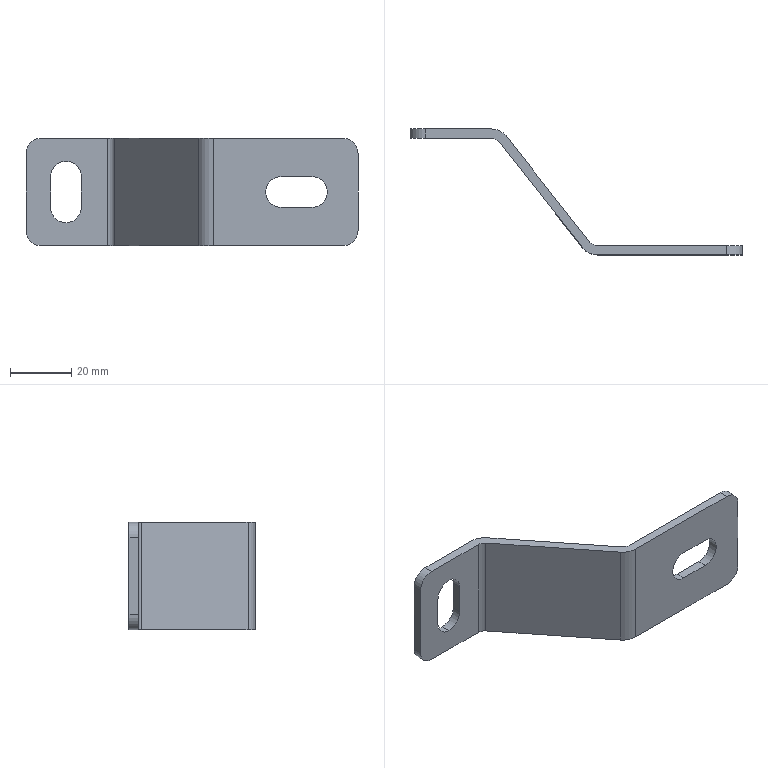Part | STEP file | VD-SYL0380DJ1006_1-4_VD-SYL0380 | 1 solid | 27 faces | box 108 x 41 x 35 mm | volume 12075 mm3 | plane 14 | cylinder 13 | commonest cylinder face diameters 10 x9 6 x2 12 x2
STEP:
#1=CARTESIAN_POINT('',(65.,-38.,-5.));
#2=VERTEX_POINT('',#1);
#3=CARTESIAN_POINT('',(55.,-38.,-5.));
#4=VERTEX_POINT('',#3);
#5=CARTESIAN_POINT('',(65.,-38.,-5.));
#6=DIRECTION('',(-1.,0.,0.));
#7=VECTOR('',#6,1000.);
#8=LINE('',#5,#7);
#9=EDGE_CURVE('',#2,#4,#8,.T.);
#10=ORIENTED_EDGE('',*,*,#9,.F.);
#11=CARTESIAN_POINT('',(65.,-35.,-5.));
#12=VERTEX_POINT('',#11);
#13=CARTESIAN_POINT('',(65.,-35.,-5.));
#14=DIRECTION('',(0.,-1.,0.));
#15=VECTOR('',#14,1000.);
#16=LINE('',#13,#15);
#17=EDGE_CURVE('',#12,#2,#16,.T.);
#18=ORIENTED_EDGE('',*,*,#17,.F.);
#19=CARTESIAN_POINT('',(55.,-35.,-5.));
#20=VERTEX_POINT('',#19);
#21=CARTESIAN_POINT('',(55.,-35.,-5.));
#22=DIRECTION('',(1.,0.,0.));
#23=VECTOR('',#22,1000.);
#24=LINE('',#21,#23);
#25=EDGE_CURVE('',#20,#12,#24,.T.);
#26=ORIENTED_EDGE('',*,*,#25,.F.);
#27=CARTESIAN_POINT('',(55.,-38.,-5.));
#28=DIRECTION('',(0.,1.,0.));
#29=VECTOR('',#28,1000.);
#30=LINE('',#27,#29);
#31=EDGE_CURVE('',#4,#20,#30,.T.);
#32=ORIENTED_EDGE('',*,*,#31,.F.);
#33=EDGE_LOOP('',(#10,#18,#26,#32));
#34=FACE_OUTER_BOUND('',#33,.T.);
#35=CARTESIAN_POINT('',(60.,-36.5,-5.));
#36=DIRECTION('',(0.,0.,1.));
#37=DIRECTION('',(1.,0.,0.));
#38=AXIS2_PLACEMENT_3D('',#35,#36,#37);
#39=PLANE('',#38);
#40=ADVANCED_FACE('',(#34),#39,.T.);
#41=CARTESIAN_POINT('',(55.,-35.,5.));
#42=VERTEX_POINT('',#41);
#43=CARTESIAN_POINT('',(55.,-38.,5.));
#44=VERTEX_POINT('',#43);
#45=CARTESIAN_POINT('',(55.,-35.,5.));
#46=DIRECTION('',(0.,-1.,0.));
#47=VECTOR('',#46,1000.);
#48=LINE('',#45,#47);
#49=EDGE_CURVE('',#42,#44,#48,.T.);
#50=ORIENTED_EDGE('',*,*,#49,.T.);
#51=CARTESIAN_POINT('',(55.,-38.,0.));
#52=DIRECTION('',(0.,1.,0.));
#53=DIRECTION('',(0.,0.,-1.));
#54=AXIS2_PLACEMENT_3D('',#51,#52,#53);
#55=CIRCLE('',#54,5.);
#56=EDGE_CURVE('',#4,#44,#55,.T.);
#57=ORIENTED_EDGE('',*,*,#56,.F.);
#58=ORIENTED_EDGE('',*,*,#31,.T.);
#59=CARTESIAN_POINT('',(55.,-35.,0.));
#60=DIRECTION('',(0.,-1.,0.));
#61=DIRECTION('',(0.,0.,1.));
#62=AXIS2_PLACEMENT_3D('',#59,#60,#61);
#63=CIRCLE('',#62,5.);
#64=EDGE_CURVE('',#42,#20,#63,.T.);
#65=ORIENTED_EDGE('',*,*,#64,.F.);
#66=EDGE_LOOP('',(#50,#57,#58,#65));
#67=FACE_OUTER_BOUND('',#66,.T.);
#68=CARTESIAN_POINT('',(55.,-36.5,0.));
#69=DIRECTION('',(0.,-1.,0.));
#70=DIRECTION('',(0.,0.,-1.));
#71=AXIS2_PLACEMENT_3D('',#68,#69,#70);
#72=CYLINDRICAL_SURFACE('',#71,5.);
#73=ADVANCED_FACE('',(#67),#72,.F.);
#74=CARTESIAN_POINT('',(65.,-38.,5.));
#75=VERTEX_POINT('',#74);
#76=CARTESIAN_POINT('',(55.,-38.,5.));
#77=DIRECTION('',(1.,0.,0.));
#78=VECTOR('',#77,1000.);
#79=LINE('',#76,#78);
#80=EDGE_CURVE('',#44,#75,#79,.T.);
#81=ORIENTED_EDGE('',*,*,#80,.F.);
#82=ORIENTED_EDGE('',*,*,#49,.F.);
#83=CARTESIAN_POINT('',(65.,-35.,5.));
#84=VERTEX_POINT('',#83);
#85=CARTESIAN_POINT('',(65.,-35.,5.));
#86=DIRECTION('',(-1.,0.,0.));
#87=VECTOR('',#86,1000.);
#88=LINE('',#85,#87);
#89=EDGE_CURVE('',#84,#42,#88,.T.);
#90=ORIENTED_EDGE('',*,*,#89,.F.);
#91=CARTESIAN_POINT('',(65.,-38.,5.));
#92=DIRECTION('',(0.,1.,0.));
#93=VECTOR('',#92,1000.);
#94=LINE('',#91,#93);
#95=EDGE_CURVE('',#75,#84,#94,.T.);
#96=ORIENTED_EDGE('',*,*,#95,.F.);
#97=EDGE_LOOP('',(#81,#82,#90,#96));
#98=FACE_OUTER_BOUND('',#97,.T.);
#99=CARTESIAN_POINT('',(60.,-36.5,5.));
#100=DIRECTION('',(0.,0.,-1.));
#101=DIRECTION('',(0.,-1.,0.));
#102=AXIS2_PLACEMENT_3D('',#99,#100,#101);
#103=PLANE('',#102);
#104=ADVANCED_FACE('',(#98),#103,.T.);
#105=ORIENTED_EDGE('',*,*,#17,.T.);
#106=CARTESIAN_POINT('',(65.,-38.,0.));
#107=DIRECTION('',(0.,1.,0.));
#108=DIRECTION('',(0.,0.,1.));
#109=AXIS2_PLACEMENT_3D('',#106,#107,#108);
#110=CIRCLE('',#109,5.);
#111=EDGE_CURVE('',#75,#2,#110,.T.);
#112=ORIENTED_EDGE('',*,*,#111,.F.);
#113=ORIENTED_EDGE('',*,*,#95,.T.);
#114=CARTESIAN_POINT('',(65.,-35.,0.));
#115=DIRECTION('',(0.,-1.,0.));
#116=DIRECTION('',(0.,0.,-1.));
#117=AXIS2_PLACEMENT_3D('',#114,#115,#116);
#118=CIRCLE('',#117,5.);
#119=EDGE_CURVE('',#12,#84,#118,.T.);
#120=ORIENTED_EDGE('',*,*,#119,.F.);
#121=EDGE_LOOP('',(#105,#112,#113,#120));
#122=FACE_OUTER_BOUND('',#121,.T.);
#123=CARTESIAN_POINT('',(65.,-36.5,0.));
#124=DIRECTION('',(0.,-1.,0.));
#125=DIRECTION('',(0.,0.,-1.));
#126=AXIS2_PLACEMENT_3D('',#123,#124,#125);
#127=CYLINDRICAL_SURFACE('',#126,5.);
#128=ADVANCED_FACE('',(#122),#127,.F.);
#129=CARTESIAN_POINT('',(75.,-38.,-17.5));
#130=VERTEX_POINT('',#129);
#131=CARTESIAN_POINT('',(80.,-38.,-12.5));
#132=VERTEX_POINT('',#131);
#133=CARTESIAN_POINT('',(75.,-38.,-12.5));
#134=DIRECTION('',(0.,-1.,0.));
#135=DIRECTION('',(0.,0.,-1.));
#136=AXIS2_PLACEMENT_3D('',#133,#134,#135);
#137=CIRCLE('',#136,5.);
#138=EDGE_CURVE('',#130,#132,#137,.T.);
#139=ORIENTED_EDGE('',*,*,#138,.F.);
#140=CARTESIAN_POINT('',(75.,-35.,-17.5));
#141=VERTEX_POINT('',#140);
#142=CARTESIAN_POINT('',(75.,-38.,-17.5));
#143=DIRECTION('',(0.,1.,0.));
#144=VECTOR('',#143,1000.);
#145=LINE('',#142,#144);
#146=EDGE_CURVE('',#130,#141,#145,.T.);
#147=ORIENTED_EDGE('',*,*,#146,.T.);
#148=CARTESIAN_POINT('',(80.,-35.,-12.5));
#149=VERTEX_POINT('',#148);
#150=CARTESIAN_POINT('',(75.,-35.,-12.5));
#151=DIRECTION('',(0.,1.,0.));
#152=DIRECTION('',(1.,0.,0.));
#153=AXIS2_PLACEMENT_3D('',#150,#151,#152);
#154=CIRCLE('',#153,5.);
#155=EDGE_CURVE('',#149,#141,#154,.T.);
#156=ORIENTED_EDGE('',*,*,#155,.F.);
#157=CARTESIAN_POINT('',(80.,-35.,-12.5));
#158=DIRECTION('',(0.,-1.,0.));
#159=VECTOR('',#158,1000.);
#160=LINE('',#157,#159);
#161=EDGE_CURVE('',#149,#132,#160,.T.);
#162=ORIENTED_EDGE('',*,*,#161,.T.);
#163=EDGE_LOOP('',(#139,#147,#156,#162));
#164=FACE_OUTER_BOUND('',#163,.T.);
#165=CARTESIAN_POINT('',(75.,61.549,-12.5));
#166=DIRECTION('',(0.,-1.,0.));
#167=DIRECTION('',(0.,0.,-1.));
#168=AXIS2_PLACEMENT_3D('',#165,#166,#167);
#169=CYLINDRICAL_SURFACE('',#168,5.);
#170=ADVANCED_FACE('',(#164),#169,.T.);
#171=CARTESIAN_POINT('',(-10.,3.,5.));
#172=VERTEX_POINT('',#171);
#173=CARTESIAN_POINT('',(-20.,3.,5.));
#174=VERTEX_POINT('',#173);
#175=CARTESIAN_POINT('',(-15.,3.,5.));
#176=DIRECTION('',(0.,-1.,0.));
#177=DIRECTION('',(1.,0.,0.));
#178=AXIS2_PLACEMENT_3D('',#175,#176,#177);
#179=CIRCLE('',#178,5.);
#180=EDGE_CURVE('',#172,#174,#179,.T.);
#181=ORIENTED_EDGE('',*,*,#180,.F.);
#182=CARTESIAN_POINT('',(-10.,0.,5.));
#183=VERTEX_POINT('',#182);
#184=CARTESIAN_POINT('',(-10.,3.,5.));
#185=DIRECTION('',(0.,-1.,0.));
#186=VECTOR('',#185,1000.);
#187=LINE('',#184,#186);
#188=EDGE_CURVE('',#172,#183,#187,.T.);
#189=ORIENTED_EDGE('',*,*,#188,.T.);
#190=CARTESIAN_POINT('',(-20.,0.,5.));
#191=VERTEX_POINT('',#190);
#192=CARTESIAN_POINT('',(-15.,0.,5.));
#193=DIRECTION('',(0.,1.,0.));
#194=DIRECTION('',(-1.,0.,0.));
#195=AXIS2_PLACEMENT_3D('',#192,#193,#194);
#196=CIRCLE('',#195,5.);
#197=EDGE_CURVE('',#191,#183,#196,.T.);
#198=ORIENTED_EDGE('',*,*,#197,.F.);
#199=CARTESIAN_POINT('',(-20.,0.,5.));
#200=DIRECTION('',(0.,1.,0.));
#201=VECTOR('',#200,1000.);
#202=LINE('',#199,#201);
#203=EDGE_CURVE('',#191,#174,#202,.T.);
#204=ORIENTED_EDGE('',*,*,#203,.T.);
#205=EDGE_LOOP('',(#181,#189,#198,#204));
#206=FACE_OUTER_BOUND('',#205,.T.);
#207=CARTESIAN_POINT('',(-15.,1.5,5.));
#208=DIRECTION('',(0.,-1.,0.));
#209=DIRECTION('',(0.,0.,-1.));
#210=AXIS2_PLACEMENT_3D('',#207,#208,#209);
#211=CYLINDRICAL_SURFACE('',#210,5.);
#212=ADVANCED_FACE('',(#206),#211,.F.);
#213=CARTESIAN_POINT('',(-20.,0.,-5.));
#214=VERTEX_POINT('',#213);
#215=CARTESIAN_POINT('',(-20.,0.,-5.));
#216=DIRECTION('',(0.,0.,1.));
#217=VECTOR('',#216,1000.);
#218=LINE('',#215,#217);
#219=EDGE_CURVE('',#214,#191,#218,.T.);
#220=ORIENTED_EDGE('',*,*,#219,.F.);
#221=CARTESIAN_POINT('',(-20.,3.,-5.));
#222=VERTEX_POINT('',#221);
#223=CARTESIAN_POINT('',(-20.,3.,-5.));
#224=DIRECTION('',(0.,-1.,0.));
#225=VECTOR('',#224,1000.);
#226=LINE('',#223,#225);
#227=EDGE_CURVE('',#222,#214,#226,.T.);
#228=ORIENTED_EDGE('',*,*,#227,.F.);
#229=CARTESIAN_POINT('',(-20.,3.,5.));
#230=DIRECTION('',(0.,0.,-1.));
#231=VECTOR('',#230,1000.);
#232=LINE('',#229,#231);
#233=EDGE_CURVE('',#174,#222,#232,.T.);
#234=ORIENTED_EDGE('',*,*,#233,.F.);
#235=ORIENTED_EDGE('',*,*,#203,.F.);
#236=EDGE_LOOP('',(#220,#228,#234,#235));
#237=FACE_OUTER_BOUND('',#236,.T.);
#238=CARTESIAN_POINT('',(-20.,1.5,0.));
#239=DIRECTION('',(1.,0.,0.));
#240=DIRECTION('',(0.,1.,0.));
#241=AXIS2_PLACEMENT_3D('',#238,#239,#240);
#242=PLANE('',#241);
#243=ADVANCED_FACE('',(#237),#242,.T.);
#244=CARTESIAN_POINT('',(-15.,3.,-10.));
#245=VERTEX_POINT('',#244);
#246=CARTESIAN_POINT('',(-15.,3.,-5.));
#247=DIRECTION('',(0.,-1.,0.));
#248=DIRECTION('',(-1.,0.,0.));
#249=AXIS2_PLACEMENT_3D('',#246,#247,#248);
#250=CIRCLE('',#249,5.);
#251=EDGE_CURVE('',#222,#245,#250,.T.);
#252=ORIENTED_EDGE('',*,*,#251,.F.);
#253=ORIENTED_EDGE('',*,*,#227,.T.);
#254=CARTESIAN_POINT('',(-15.,0.,-10.));
#255=VERTEX_POINT('',#254);
#256=CARTESIAN_POINT('',(-15.,0.,-5.));
#257=DIRECTION('',(0.,1.,0.));
#258=DIRECTION('',(0.,0.,-1.));
#259=AXIS2_PLACEMENT_3D('',#256,#257,#258);
#260=CIRCLE('',#259,5.);
#261=EDGE_CURVE('',#255,#214,#260,.T.);
#262=ORIENTED_EDGE('',*,*,#261,.F.);
#263=CARTESIAN_POINT('',(-15.,0.,-10.));
#264=DIRECTION('',(0.,1.,0.));
#265=VECTOR('',#264,1000.);
#266=LINE('',#263,#265);
#267=EDGE_CURVE('',#255,#245,#266,.T.);
#268=ORIENTED_EDGE('',*,*,#267,.T.);
#269=EDGE_LOOP('',(#252,#253,#262,#268));
#270=FACE_OUTER_BOUND('',#269,.T.);
#271=CARTESIAN_POINT('',(-15.,1.5,-5.));
#272=DIRECTION('',(0.,-1.,0.));
#273=DIRECTION('',(0.,0.,-1.));
#274=AXIS2_PLACEMENT_3D('',#271,#272,#273);
#275=CYLINDRICAL_SURFACE('',#274,5.);
#276=ADVANCED_FACE('',(#270),#275,.F.);
#277=ORIENTED_EDGE('',*,*,#267,.F.);
#278=CARTESIAN_POINT('',(-10.,0.,-5.));
#279=VERTEX_POINT('',#278);
#280=CARTESIAN_POINT('',(-15.,0.,-5.));
#281=DIRECTION('',(0.,1.,0.));
#282=DIRECTION('',(1.,0.,0.));
#283=AXIS2_PLACEMENT_3D('',#280,#281,#282);
#284=CIRCLE('',#283,5.);
#285=EDGE_CURVE('',#279,#255,#284,.T.);
#286=ORIENTED_EDGE('',*,*,#285,.F.);
#287=CARTESIAN_POINT('',(-10.,3.,-5.));
#288=VERTEX_POINT('',#287);
#289=CARTESIAN_POINT('',(-10.,0.,-5.));
#290=DIRECTION('',(0.,1.,0.));
#291=VECTOR('',#290,1000.);
#292=LINE('',#289,#291);
#293=EDGE_CURVE('',#279,#288,#292,.T.);
#294=ORIENTED_EDGE('',*,*,#293,.T.);
#295=CARTESIAN_POINT('',(-15.,3.,-5.));
#296=DIRECTION('',(0.,-1.,0.));
#297=DIRECTION('',(0.,0.,-1.));
#298=AXIS2_PLACEMENT_3D('',#295,#296,#297);
#299=CIRCLE('',#298,5.);
#300=EDGE_CURVE('',#245,#288,#299,.T.);
#301=ORIENTED_EDGE('',*,*,#300,.F.);
#302=EDGE_LOOP('',(#277,#286,#294,#301));
#303=FACE_OUTER_BOUND('',#302,.T.);
#304=CARTESIAN_POINT('',(-15.,1.5,-5.));
#305=DIRECTION('',(0.,-1.,0.));
#306=DIRECTION('',(0.,0.,-1.));
#307=AXIS2_PLACEMENT_3D('',#304,#305,#306);
#308=CYLINDRICAL_SURFACE('',#307,5.);
#309=ADVANCED_FACE('',(#303),#308,.F.);
#310=CARTESIAN_POINT('',(-10.,0.,5.));
#311=DIRECTION('',(0.,0.,-1.));
#312=VECTOR('',#311,1000.);
#313=LINE('',#310,#312);
#314=EDGE_CURVE('',#183,#279,#313,.T.);
#315=ORIENTED_EDGE('',*,*,#314,.F.);
#316=ORIENTED_EDGE('',*,*,#188,.F.);
#317=CARTESIAN_POINT('',(-10.,3.,-5.));
#318=DIRECTION('',(0.,0.,1.));
#319=VECTOR('',#318,1000.);
#320=LINE('',#317,#319);
#321=EDGE_CURVE('',#288,#172,#320,.T.);
#322=ORIENTED_EDGE('',*,*,#321,.F.);
#323=ORIENTED_EDGE('',*,*,#293,.F.);
#324=EDGE_LOOP('',(#315,#316,#322,#323));
#325=FACE_OUTER_BOUND('',#324,.T.);
#326=CARTESIAN_POINT('',(-10.,1.5,0.));
#327=DIRECTION('',(-1.,0.,0.));
#328=DIRECTION('',(0.,0.,1.));
#329=AXIS2_PLACEMENT_3D('',#326,#327,#328);
#330=PLANE('',#329);
#331=ADVANCED_FACE('',(#325),#330,.T.);
#332=CARTESIAN_POINT('',(-28.,0.,-12.5));
#333=VERTEX_POINT('',#332);
#334=CARTESIAN_POINT('',(-23.,0.,-17.5));
#335=VERTEX_POINT('',#334);
#336=CARTESIAN_POINT('',(-23.,0.,-12.5));
#337=DIRECTION('',(0.,-1.,0.));
#338=DIRECTION('',(-1.,0.,0.));
#339=AXIS2_PLACEMENT_3D('',#336,#337,#338);
#340=CIRCLE('',#339,5.);
#341=EDGE_CURVE('',#333,#335,#340,.T.);
#342=ORIENTED_EDGE('',*,*,#341,.F.);
#343=CARTESIAN_POINT('',(-28.,3.,-12.5));
#344=VERTEX_POINT('',#343);
#345=CARTESIAN_POINT('',(-28.,0.,-12.5));
#346=DIRECTION('',(0.,1.,0.));
#347=VECTOR('',#346,1000.);
#348=LINE('',#345,#347);
#349=EDGE_CURVE('',#333,#344,#348,.T.);
#350=ORIENTED_EDGE('',*,*,#349,.T.);
#351=CARTESIAN_POINT('',(-23.,3.,-17.5));
#352=VERTEX_POINT('',#351);
#353=CARTESIAN_POINT('',(-23.,3.,-12.5));
#354=DIRECTION('',(0.,1.,0.));
#355=DIRECTION('',(0.,0.,-1.));
#356=AXIS2_PLACEMENT_3D('',#353,#354,#355);
#357=CIRCLE('',#356,5.);
#358=EDGE_CURVE('',#352,#344,#357,.T.);
#359=ORIENTED_EDGE('',*,*,#358,.F.);
#360=CARTESIAN_POINT('',(-23.,3.,-17.5));
#361=DIRECTION('',(0.,-1.,0.));
#362=VECTOR('',#361,1000.);
#363=LINE('',#360,#362);
#364=EDGE_CURVE('',#352,#335,#363,.T.);
#365=ORIENTED_EDGE('',*,*,#364,.T.);
#366=EDGE_LOOP('',(#342,#350,#359,#365));
#367=FACE_OUTER_BOUND('',#366,.T.);
#368=CARTESIAN_POINT('',(-23.,61.549,-12.5));
#369=DIRECTION('',(0.,-1.,0.));
#370=DIRECTION('',(0.,0.,-1.));
#371=AXIS2_PLACEMENT_3D('',#368,#369,#370);
#372=CYLINDRICAL_SURFACE('',#371,5.);
#373=ADVANCED_FACE('',(#367),#372,.T.);
#374=ORIENTED_EDGE('',*,*,#180,.T.);
#375=ORIENTED_EDGE('',*,*,#233,.T.);
#376=ORIENTED_EDGE('',*,*,#251,.T.);
#377=ORIENTED_EDGE('',*,*,#300,.T.);
#378=ORIENTED_EDGE('',*,*,#321,.T.);
#379=EDGE_LOOP('',(#374,#375,#376,#377,#378));
#380=FACE_BOUND('',#379,.T.);
#381=CARTESIAN_POINT('',(-23.,3.,17.5));
#382=VERTEX_POINT('',#381);
#383=CARTESIAN_POINT('',(-1.454,3.,17.5));
#384=VERTEX_POINT('',#383);
#385=CARTESIAN_POINT('',(-23.,3.,17.5));
#386=DIRECTION('',(1.,0.,0.));
#387=VECTOR('',#386,1000.);
#388=LINE('',#385,#387);
#389=EDGE_CURVE('',#382,#384,#388,.T.);
#390=ORIENTED_EDGE('',*,*,#389,.T.);
#391=CARTESIAN_POINT('',(-1.454,3.,-17.5));
#392=VERTEX_POINT('',#391);
#393=CARTESIAN_POINT('',(-1.454,3.,-17.5));
#394=DIRECTION('',(0.,0.,1.));
#395=VECTOR('',#394,1000.);
#396=LINE('',#393,#395);
#397=EDGE_CURVE('',#392,#384,#396,.T.);
#398=ORIENTED_EDGE('',*,*,#397,.F.);
#399=CARTESIAN_POINT('',(-1.454,3.,-17.5));
#400=DIRECTION('',(-1.,0.,0.));
#401=VECTOR('',#400,1000.);
#402=LINE('',#399,#401);
#403=EDGE_CURVE('',#392,#352,#402,.T.);
#404=ORIENTED_EDGE('',*,*,#403,.T.);
#405=ORIENTED_EDGE('',*,*,#358,.T.);
#406=CARTESIAN_POINT('',(-28.,3.,12.5));
#407=VERTEX_POINT('',#406);
#408=CARTESIAN_POINT('',(-28.,3.,-12.5));
#409=DIRECTION('',(0.,0.,1.));
#410=VECTOR('',#409,1000.);
#411=LINE('',#408,#410);
#412=EDGE_CURVE('',#344,#407,#411,.T.);
#413=ORIENTED_EDGE('',*,*,#412,.T.);
#414=CARTESIAN_POINT('',(-23.,3.,12.5));
#415=DIRECTION('',(0.,1.,0.));
#416=DIRECTION('',(-1.,0.,0.));
#417=AXIS2_PLACEMENT_3D('',#414,#415,#416);
#418=CIRCLE('',#417,5.);
#419=EDGE_CURVE('',#407,#382,#418,.T.);
#420=ORIENTED_EDGE('',*,*,#419,.T.);
#421=EDGE_LOOP('',(#390,#398,#404,#405,#413,#420));
#422=FACE_OUTER_BOUND('',#421,.T.);
#423=CARTESIAN_POINT('',(-28.,3.,-17.5));
#424=DIRECTION('',(0.,-1.,0.));
#425=DIRECTION('',(0.,0.,-1.));
#426=AXIS2_PLACEMENT_3D('',#423,#424,#425);
#427=PLANE('',#426);
#428=ADVANCED_FACE('',(#380,#422),#427,.F.);
#429=CARTESIAN_POINT('',(-23.,0.,17.5));
#430=VERTEX_POINT('',#429);
#431=CARTESIAN_POINT('',(-28.,0.,12.5));
#432=VERTEX_POINT('',#431);
#433=CARTESIAN_POINT('',(-23.,0.,12.5));
#434=DIRECTION('',(0.,-1.,0.));
#435=DIRECTION('',(0.,0.,1.));
#436=AXIS2_PLACEMENT_3D('',#433,#434,#435);
#437=CIRCLE('',#436,5.);
#438=EDGE_CURVE('',#430,#432,#437,.T.);
#439=ORIENTED_EDGE('',*,*,#438,.F.);
#440=CARTESIAN_POINT('',(-23.,0.,17.5));
#441=DIRECTION('',(0.,1.,0.));
#442=VECTOR('',#441,1000.);
#443=LINE('',#440,#442);
#444=EDGE_CURVE('',#430,#382,#443,.T.);
#445=ORIENTED_EDGE('',*,*,#444,.T.);
#446=ORIENTED_EDGE('',*,*,#419,.F.);
#447=CARTESIAN_POINT('',(-28.,3.,12.5));
#448=DIRECTION('',(0.,-1.,0.));
#449=VECTOR('',#448,1000.);
#450=LINE('',#447,#449);
#451=EDGE_CURVE('',#407,#432,#450,.T.);
#452=ORIENTED_EDGE('',*,*,#451,.T.);
#453=EDGE_LOOP('',(#439,#445,#446,#452));
#454=FACE_OUTER_BOUND('',#453,.T.);
#455=CARTESIAN_POINT('',(-23.,61.549,12.5));
#456=DIRECTION('',(0.,-1.,0.));
#457=DIRECTION('',(0.,0.,-1.));
#458=AXIS2_PLACEMENT_3D('',#455,#456,#457);
#459=CYLINDRICAL_SURFACE('',#458,5.);
#460=ADVANCED_FACE('',(#454),#459,.T.);
#461=ORIENTED_EDGE('',*,*,#412,.F.);
#462=ORIENTED_EDGE('',*,*,#349,.F.);
#463=CARTESIAN_POINT('',(-28.,0.,-12.5));
#464=DIRECTION('',(0.,0.,1.));
#465=VECTOR('',#464,1000.);
#466=LINE('',#463,#465);
#467=EDGE_CURVE('',#333,#432,#466,.T.);
#468=ORIENTED_EDGE('',*,*,#467,.T.);
#469=ORIENTED_EDGE('',*,*,#451,.F.);
#470=EDGE_LOOP('',(#461,#462,#468,#469));
#471=FACE_OUTER_BOUND('',#470,.T.);
#472=CARTESIAN_POINT('',(-28.,1.5,0.));
#473=DIRECTION('',(1.,0.,0.));
#474=DIRECTION('',(0.,1.,0.));
#475=AXIS2_PLACEMENT_3D('',#472,#473,#474);
#476=PLANE('',#475);
#477=ADVANCED_FACE('',(#471),#476,.F.);
#478=ORIENTED_EDGE('',*,*,#261,.T.);
#479=ORIENTED_EDGE('',*,*,#219,.T.);
#480=ORIENTED_EDGE('',*,*,#197,.T.);
#481=ORIENTED_EDGE('',*,*,#314,.T.);
#482=ORIENTED_EDGE('',*,*,#285,.T.);
#483=EDGE_LOOP('',(#478,#479,#480,#481,#482));
#484=FACE_BOUND('',#483,.T.);
#485=ORIENTED_EDGE('',*,*,#341,.T.);
#486=CARTESIAN_POINT('',(-1.454,0.,-17.5));
#487=VERTEX_POINT('',#486);
#488=CARTESIAN_POINT('',(-23.,0.,-17.5));
#489=DIRECTION('',(1.,0.,0.));
#490=VECTOR('',#489,1000.);
#491=LINE('',#488,#490);
#492=EDGE_CURVE('',#335,#487,#491,.T.);
#493=ORIENTED_EDGE('',*,*,#492,.T.);
#494=CARTESIAN_POINT('',(-1.454,0.,17.5));
#495=VERTEX_POINT('',#494);
#496=CARTESIAN_POINT('',(-1.454,0.,17.5));
#497=DIRECTION('',(0.,0.,-1.));
#498=VECTOR('',#497,1000.);
#499=LINE('',#496,#498);
#500=EDGE_CURVE('',#495,#487,#499,.T.);
#501=ORIENTED_EDGE('',*,*,#500,.F.);
#502=CARTESIAN_POINT('',(-23.,0.,17.5));
#503=DIRECTION('',(1.,0.,0.));
#504=VECTOR('',#503,1000.);
#505=LINE('',#502,#504);
#506=EDGE_CURVE('',#430,#495,#505,.T.);
#507=ORIENTED_EDGE('',*,*,#506,.F.);
#508=ORIENTED_EDGE('',*,*,#438,.T.);
#509=ORIENTED_EDGE('',*,*,#467,.F.);
#510=EDGE_LOOP('',(#485,#493,#501,#507,#508,#509));
#511=FACE_OUTER_BOUND('',#510,.T.);
#512=CARTESIAN_POINT('',(-28.,0.,-17.5));
#513=DIRECTION('',(0.,-1.,0.));
#514=DIRECTION('',(0.,0.,-1.));
#515=AXIS2_PLACEMENT_3D('',#512,#513,#514);
#516=PLANE('',#515);
#517=ADVANCED_FACE('',(#484,#511),#516,.T.);
#518=CARTESIAN_POINT('',(0.9008,-1.141,-17.5));
#519=VERTEX_POINT('',#518);
#520=CARTESIAN_POINT('',(-1.454,-3.,-17.5));
#521=DIRECTION('',(0.,0.,1.));
#522=DIRECTION('',(0.7849,0.6196,0.));
#523=AXIS2_PLACEMENT_3D('',#520,#521,#522);
#524=CIRCLE('',#523,3.);
#525=EDGE_CURVE('',#519,#487,#524,.T.);
#526=ORIENTED_EDGE('',*,*,#525,.F.);
#527=CARTESIAN_POINT('',(0.9008,-1.141,17.5));
#528=VERTEX_POINT('',#527);
#529=CARTESIAN_POINT('',(0.9008,-1.141,-17.5));
#530=DIRECTION('',(0.,0.,1.));
#531=VECTOR('',#530,1000.);
#532=LINE('',#529,#531);
#533=EDGE_CURVE('',#519,#528,#532,.T.);
#534=ORIENTED_EDGE('',*,*,#533,.T.);
#535=CARTESIAN_POINT('',(-1.454,-3.,17.5));
#536=DIRECTION('',(0.,0.,-1.));
#537=DIRECTION('',(0.,1.,0.));
#538=AXIS2_PLACEMENT_3D('',#535,#536,#537);
#539=CIRCLE('',#538,3.);
#540=EDGE_CURVE('',#495,#528,#539,.T.);
#541=ORIENTED_EDGE('',*,*,#540,.F.);
#542=ORIENTED_EDGE('',*,*,#500,.T.);
#543=EDGE_LOOP('',(#526,#534,#541,#542));
#544=FACE_OUTER_BOUND('',#543,.T.);
#545=CARTESIAN_POINT('',(-1.454,-3.,-131.142));
#546=DIRECTION('',(0.,0.,1.));
#547=DIRECTION('',(1.,0.,0.));
#548=AXIS2_PLACEMENT_3D('',#545,#546,#547);
#549=CYLINDRICAL_SURFACE('',#548,3.);
#550=ADVANCED_FACE('',(#544),#549,.F.);
#551=CARTESIAN_POINT('',(28.198,-35.718,17.5));
#552=VERTEX_POINT('',#551);
#553=CARTESIAN_POINT('',(28.198,-35.718,-17.5));
#554=VERTEX_POINT('',#553);
#555=CARTESIAN_POINT('',(28.198,-35.718,17.5));
#556=DIRECTION('',(0.,0.,-1.));
#557=VECTOR('',#556,1000.);
#558=LINE('',#555,#557);
#559=EDGE_CURVE('',#552,#554,#558,.T.);
#560=ORIENTED_EDGE('',*,*,#559,.F.);
#561=CARTESIAN_POINT('',(0.9008,-1.141,17.5));
#562=DIRECTION('',(0.6196,-0.7849,0.));
#563=VECTOR('',#562,1000.);
#564=LINE('',#561,#563);
#565=EDGE_CURVE('',#528,#552,#564,.T.);
#566=ORIENTED_EDGE('',*,*,#565,.F.);
#567=ORIENTED_EDGE('',*,*,#533,.F.);
#568=CARTESIAN_POINT('',(28.198,-35.718,-17.5));
#569=DIRECTION('',(-0.6196,0.7849,0.));
#570=VECTOR('',#569,1000.);
#571=LINE('',#568,#570);
#572=EDGE_CURVE('',#554,#519,#571,.T.);
#573=ORIENTED_EDGE('',*,*,#572,.F.);
#574=EDGE_LOOP('',(#560,#566,#567,#573));
#575=FACE_OUTER_BOUND('',#574,.T.);
#576=CARTESIAN_POINT('',(0.,0.,-17.5));
#577=DIRECTION('',(-0.7849,-0.6196,0.));
#578=DIRECTION('',(-0.6196,0.7849,0.));
#579=AXIS2_PLACEMENT_3D('',#576,#577,#578);
#580=PLANE('',#579);
#581=ADVANCED_FACE('',(#575),#580,.T.);
#582=ORIENTED_EDGE('',*,*,#559,.T.);
#583=CARTESIAN_POINT('',(32.908,-38.,-17.5));
#584=VERTEX_POINT('',#583);
#585=CARTESIAN_POINT('',(32.908,-32.,-17.5));
#586=DIRECTION('',(0.,0.,-1.));
#587=DIRECTION('',(0.,-1.,0.));
#588=AXIS2_PLACEMENT_3D('',#585,#586,#587);
#589=CIRCLE('',#588,6.);
#590=EDGE_CURVE('',#584,#554,#589,.T.);
#591=ORIENTED_EDGE('',*,*,#590,.F.);
#592=CARTESIAN_POINT('',(32.908,-38.,17.5));
#593=VERTEX_POINT('',#592);
#594=CARTESIAN_POINT('',(32.908,-38.,-17.5));
#595=DIRECTION('',(0.,0.,1.));
#596=VECTOR('',#595,1000.);
#597=LINE('',#594,#596);
#598=EDGE_CURVE('',#584,#593,#597,.T.);
#599=ORIENTED_EDGE('',*,*,#598,.T.);
#600=CARTESIAN_POINT('',(32.908,-32.,17.5));
#601=DIRECTION('',(0.,0.,1.));
#602=DIRECTION('',(-0.7849,-0.6196,0.));
#603=AXIS2_PLACEMENT_3D('',#600,#601,#602);
#604=CIRCLE('',#603,6.);
#605=EDGE_CURVE('',#552,#593,#604,.T.);
#606=ORIENTED_EDGE('',*,*,#605,.F.);
#607=EDGE_LOOP('',(#582,#591,#599,#606));
#608=FACE_OUTER_BOUND('',#607,.T.);
#609=CARTESIAN_POINT('',(32.908,-32.,131.142));
#610=DIRECTION('',(0.,0.,-1.));
#611=DIRECTION('',(-1.,0.,0.));
#612=AXIS2_PLACEMENT_3D('',#609,#610,#611);
#613=CYLINDRICAL_SURFACE('',#612,6.);
#614=ADVANCED_FACE('',(#608),#613,.T.);
#615=ORIENTED_EDGE('',*,*,#9,.T.);
#616=ORIENTED_EDGE('',*,*,#56,.T.);
#617=ORIENTED_EDGE('',*,*,#80,.T.);
#618=ORIENTED_EDGE('',*,*,#111,.T.);
#619=EDGE_LOOP('',(#615,#616,#617,#618));
#620=FACE_BOUND('',#619,.T.);
#621=ORIENTED_EDGE('',*,*,#138,.T.);
#622=CARTESIAN_POINT('',(80.,-38.,12.5));
#623=VERTEX_POINT('',#622);
#624=CARTESIAN_POINT('',(80.,-38.,-12.5));
#625=DIRECTION('',(0.,0.,1.));
#626=VECTOR('',#625,1000.);
#627=LINE('',#624,#626);
#628=EDGE_CURVE('',#132,#623,#627,.T.);
#629=ORIENTED_EDGE('',*,*,#628,.T.);
#630=CARTESIAN_POINT('',(75.,-38.,17.5));
#631=VERTEX_POINT('',#630);
#632=CARTESIAN_POINT('',(75.,-38.,12.5));
#633=DIRECTION('',(0.,-1.,0.));
#634=DIRECTION('',(1.,0.,0.));
#635=AXIS2_PLACEMENT_3D('',#632,#633,#634);
#636=CIRCLE('',#635,5.);
#637=EDGE_CURVE('',#623,#631,#636,.T.);
#638=ORIENTED_EDGE('',*,*,#637,.T.);
#639=CARTESIAN_POINT('',(32.908,-38.,17.5));
#640=DIRECTION('',(1.,0.,0.));
#641=VECTOR('',#640,1000.);
#642=LINE('',#639,#641);
#643=EDGE_CURVE('',#593,#631,#642,.T.);
#644=ORIENTED_EDGE('',*,*,#643,.F.);
#645=ORIENTED_EDGE('',*,*,#598,.F.);
#646=CARTESIAN_POINT('',(32.908,-38.,-17.5));
#647=DIRECTION('',(1.,0.,0.));
#648=VECTOR('',#647,1000.);
#649=LINE('',#646,#648);
#650=EDGE_CURVE('',#584,#130,#649,.T.);
#651=ORIENTED_EDGE('',*,*,#650,.T.);
#652=EDGE_LOOP('',(#621,#629,#638,#644,#645,#651));
#653=FACE_OUTER_BOUND('',#652,.T.);
#654=CARTESIAN_POINT('',(30.,-38.,-17.5));
#655=DIRECTION('',(0.,-1.,0.));
#656=DIRECTION('',(0.,0.,-1.));
#657=AXIS2_PLACEMENT_3D('',#654,#655,#656);
#658=PLANE('',#657);
#659=ADVANCED_FACE('',(#620,#653),#658,.T.);
#660=ORIENTED_EDGE('',*,*,#161,.F.);
#661=CARTESIAN_POINT('',(80.,-35.,12.5));
#662=VERTEX_POINT('',#661);
#663=CARTESIAN_POINT('',(80.,-35.,12.5));
#664=DIRECTION('',(0.,0.,-1.));
#665=VECTOR('',#664,1000.);
#666=LINE('',#663,#665);
#667=EDGE_CURVE('',#662,#149,#666,.T.);
#668=ORIENTED_EDGE('',*,*,#667,.F.);
#669=CARTESIAN_POINT('',(80.,-38.,12.5));
#670=DIRECTION('',(0.,1.,0.));
#671=VECTOR('',#670,1000.);
#672=LINE('',#669,#671);
#673=EDGE_CURVE('',#623,#662,#672,.T.);
#674=ORIENTED_EDGE('',*,*,#673,.F.);
#675=ORIENTED_EDGE('',*,*,#628,.F.);
#676=EDGE_LOOP('',(#660,#668,#674,#675));
#677=FACE_OUTER_BOUND('',#676,.T.);
#678=CARTESIAN_POINT('',(80.,-36.5,0.));
#679=DIRECTION('',(1.,0.,0.));
#680=DIRECTION('',(0.,1.,0.));
#681=AXIS2_PLACEMENT_3D('',#678,#679,#680);
#682=PLANE('',#681);
#683=ADVANCED_FACE('',(#677),#682,.T.);
#684=ORIENTED_EDGE('',*,*,#637,.F.);
#685=ORIENTED_EDGE('',*,*,#673,.T.);
#686=CARTESIAN_POINT('',(75.,-35.,17.5));
#687=VERTEX_POINT('',#686);
#688=CARTESIAN_POINT('',(75.,-35.,12.5));
#689=DIRECTION('',(0.,1.,0.));
#690=DIRECTION('',(0.,0.,1.));
#691=AXIS2_PLACEMENT_3D('',#688,#689,#690);
#692=CIRCLE('',#691,5.);
#693=EDGE_CURVE('',#687,#662,#692,.T.);
#694=ORIENTED_EDGE('',*,*,#693,.F.);
#695=CARTESIAN_POINT('',(75.,-35.,17.5));
#696=DIRECTION('',(0.,-1.,0.));
#697=VECTOR('',#696,1000.);
#698=LINE('',#695,#697);
#699=EDGE_CURVE('',#687,#631,#698,.T.);
#700=ORIENTED_EDGE('',*,*,#699,.T.);
#701=EDGE_LOOP('',(#684,#685,#694,#700));
#702=FACE_OUTER_BOUND('',#701,.T.);
#703=CARTESIAN_POINT('',(75.,61.549,12.5));
#704=DIRECTION('',(0.,-1.,0.));
#705=DIRECTION('',(0.,0.,-1.));
#706=AXIS2_PLACEMENT_3D('',#703,#704,#705);
#707=CYLINDRICAL_SURFACE('',#706,5.);
#708=ADVANCED_FACE('',(#702),#707,.T.);
#709=CARTESIAN_POINT('',(3.255,0.7179,17.5));
#710=VERTEX_POINT('',#709);
#711=CARTESIAN_POINT('',(-1.454,-3.,17.5));
#712=DIRECTION('',(0.,0.,1.));
#713=DIRECTION('',(0.7849,0.6196,0.));
#714=AXIS2_PLACEMENT_3D('',#711,#712,#713);
#715=CIRCLE('',#714,6.);
#716=EDGE_CURVE('',#710,#384,#715,.T.);
#717=ORIENTED_EDGE('',*,*,#716,.T.);
#718=ORIENTED_EDGE('',*,*,#389,.F.);
#719=ORIENTED_EDGE('',*,*,#444,.F.);
#720=ORIENTED_EDGE('',*,*,#506,.T.);
#721=ORIENTED_EDGE('',*,*,#540,.T.);
#722=ORIENTED_EDGE('',*,*,#565,.T.);
#723=ORIENTED_EDGE('',*,*,#605,.T.);
#724=ORIENTED_EDGE('',*,*,#643,.T.);
#725=ORIENTED_EDGE('',*,*,#699,.F.);
#726=CARTESIAN_POINT('',(32.908,-35.,17.5));
#727=VERTEX_POINT('',#726);
#728=CARTESIAN_POINT('',(32.908,-35.,17.5));
#729=DIRECTION('',(1.,0.,0.));
#730=VECTOR('',#729,1000.);
#731=LINE('',#728,#730);
#732=EDGE_CURVE('',#727,#687,#731,.T.);
#733=ORIENTED_EDGE('',*,*,#732,.F.);
#734=CARTESIAN_POINT('',(30.553,-33.859,17.5));
#735=VERTEX_POINT('',#734);
#736=CARTESIAN_POINT('',(32.908,-32.,17.5));
#737=DIRECTION('',(0.,0.,-1.));
#738=DIRECTION('',(0.,-1.,0.));
#739=AXIS2_PLACEMENT_3D('',#736,#737,#738);
#740=CIRCLE('',#739,3.);
#741=EDGE_CURVE('',#727,#735,#740,.T.);
#742=ORIENTED_EDGE('',*,*,#741,.T.);
#743=CARTESIAN_POINT('',(30.553,-33.859,17.5));
#744=DIRECTION('',(-0.6196,0.7849,0.));
#745=VECTOR('',#744,1000.);
#746=LINE('',#743,#745);
#747=EDGE_CURVE('',#735,#710,#746,.T.);
#748=ORIENTED_EDGE('',*,*,#747,.T.);
#749=EDGE_LOOP('',(#717,#718,#719,#720,#721,#722,#723,#724,#725,#733,#742,#748));
#750=FACE_OUTER_BOUND('',#749,.T.);
#751=CARTESIAN_POINT('',(15.727,-17.5,17.5));
#752=DIRECTION('',(0.,0.,-1.));
#753=DIRECTION('',(0.,-1.,0.));
#754=AXIS2_PLACEMENT_3D('',#751,#752,#753);
#755=PLANE('',#754);
#756=ADVANCED_FACE('',(#750),#755,.F.);
#757=CARTESIAN_POINT('',(3.255,0.7179,-17.5));
#758=VERTEX_POINT('',#757);
#759=CARTESIAN_POINT('',(3.255,0.7179,17.5));
#760=DIRECTION('',(0.,0.,-1.));
#761=VECTOR('',#760,1000.);
#762=LINE('',#759,#761);
#763=EDGE_CURVE('',#710,#758,#762,.T.);
#764=ORIENTED_EDGE('',*,*,#763,.T.);
#765=CARTESIAN_POINT('',(-1.454,-3.,-17.5));
#766=DIRECTION('',(0.,0.,-1.));
#767=DIRECTION('',(0.,1.,0.));
#768=AXIS2_PLACEMENT_3D('',#765,#766,#767);
#769=CIRCLE('',#768,6.);
#770=EDGE_CURVE('',#392,#758,#769,.T.);
#771=ORIENTED_EDGE('',*,*,#770,.F.);
#772=ORIENTED_EDGE('',*,*,#397,.T.);
#773=ORIENTED_EDGE('',*,*,#716,.F.);
#774=EDGE_LOOP('',(#764,#771,#772,#773));
#775=FACE_OUTER_BOUND('',#774,.T.);
#776=CARTESIAN_POINT('',(-1.454,-3.,-131.142));
#777=DIRECTION('',(0.,0.,1.));
#778=DIRECTION('',(1.,0.,0.));
#779=AXIS2_PLACEMENT_3D('',#776,#777,#778);
#780=CYLINDRICAL_SURFACE('',#779,6.);
#781=ADVANCED_FACE('',(#775),#780,.T.);
#782=ORIENTED_EDGE('',*,*,#747,.F.);
#783=CARTESIAN_POINT('',(30.553,-33.859,-17.5));
#784=VERTEX_POINT('',#783);
#785=CARTESIAN_POINT('',(30.553,-33.859,-17.5));
#786=DIRECTION('',(0.,0.,1.));
#787=VECTOR('',#786,1000.);
#788=LINE('',#785,#787);
#789=EDGE_CURVE('',#784,#735,#788,.T.);
#790=ORIENTED_EDGE('',*,*,#789,.F.);
#791=CARTESIAN_POINT('',(3.255,0.7179,-17.5));
#792=DIRECTION('',(0.6196,-0.7849,0.));
#793=VECTOR('',#792,1000.);
#794=LINE('',#791,#793);
#795=EDGE_CURVE('',#758,#784,#794,.T.);
#796=ORIENTED_EDGE('',*,*,#795,.F.);
#797=ORIENTED_EDGE('',*,*,#763,.F.);
#798=EDGE_LOOP('',(#782,#790,#796,#797));
#799=FACE_OUTER_BOUND('',#798,.T.);
#800=CARTESIAN_POINT('',(2.355,1.859,-17.5));
#801=DIRECTION('',(-0.7849,-0.6196,0.));
#802=DIRECTION('',(-0.6196,0.7849,0.));
#803=AXIS2_PLACEMENT_3D('',#800,#801,#802);
#804=PLANE('',#803);
#805=ADVANCED_FACE('',(#799),#804,.F.);
#806=CARTESIAN_POINT('',(32.908,-35.,-17.5));
#807=VERTEX_POINT('',#806);
#808=CARTESIAN_POINT('',(32.908,-32.,-17.5));
#809=DIRECTION('',(0.,0.,1.));
#810=DIRECTION('',(-0.7849,-0.6196,0.));
#811=AXIS2_PLACEMENT_3D('',#808,#809,#810);
#812=CIRCLE('',#811,3.);
#813=EDGE_CURVE('',#784,#807,#812,.T.);
#814=ORIENTED_EDGE('',*,*,#813,.T.);
#815=CARTESIAN_POINT('',(75.,-35.,-17.5));
#816=DIRECTION('',(-1.,0.,0.));
#817=VECTOR('',#816,1000.);
#818=LINE('',#815,#817);
#819=EDGE_CURVE('',#141,#807,#818,.T.);
#820=ORIENTED_EDGE('',*,*,#819,.F.);
#821=ORIENTED_EDGE('',*,*,#146,.F.);
#822=ORIENTED_EDGE('',*,*,#650,.F.);
#823=ORIENTED_EDGE('',*,*,#590,.T.);
#824=ORIENTED_EDGE('',*,*,#572,.T.);
#825=ORIENTED_EDGE('',*,*,#525,.T.);
#826=ORIENTED_EDGE('',*,*,#492,.F.);
#827=ORIENTED_EDGE('',*,*,#364,.F.);
#828=ORIENTED_EDGE('',*,*,#403,.F.);
#829=ORIENTED_EDGE('',*,*,#770,.T.);
#830=ORIENTED_EDGE('',*,*,#795,.T.);
#831=EDGE_LOOP('',(#814,#820,#821,#822,#823,#824,#825,#826,#827,#828,#829,#830));
#832=FACE_OUTER_BOUND('',#831,.T.);
#833=CARTESIAN_POINT('',(15.727,-17.5,-17.5));
#834=DIRECTION('',(0.,0.,-1.));
#835=DIRECTION('',(0.,-1.,0.));
#836=AXIS2_PLACEMENT_3D('',#833,#834,#835);
#837=PLANE('',#836);
#838=ADVANCED_FACE('',(#832),#837,.T.);
#839=ORIENTED_EDGE('',*,*,#64,.T.);
#840=ORIENTED_EDGE('',*,*,#25,.T.);
#841=ORIENTED_EDGE('',*,*,#119,.T.);
#842=ORIENTED_EDGE('',*,*,#89,.T.);
#843=EDGE_LOOP('',(#839,#840,#841,#842));
#844=FACE_BOUND('',#843,.T.);
#845=ORIENTED_EDGE('',*,*,#732,.T.);
#846=ORIENTED_EDGE('',*,*,#693,.T.);
#847=ORIENTED_EDGE('',*,*,#667,.T.);
#848=ORIENTED_EDGE('',*,*,#155,.T.);
#849=ORIENTED_EDGE('',*,*,#819,.T.);
#850=CARTESIAN_POINT('',(32.908,-35.,17.5));
#851=DIRECTION('',(0.,0.,-1.));
#852=VECTOR('',#851,1000.);
#853=LINE('',#850,#852);
#854=EDGE_CURVE('',#727,#807,#853,.T.);
#855=ORIENTED_EDGE('',*,*,#854,.F.);
#856=EDGE_LOOP('',(#845,#846,#847,#848,#849,#855));
#857=FACE_OUTER_BOUND('',#856,.T.);
#858=CARTESIAN_POINT('',(30.,-35.,-17.5));
#859=DIRECTION('',(0.,-1.,0.));
#860=DIRECTION('',(0.,0.,-1.));
#861=AXIS2_PLACEMENT_3D('',#858,#859,#860);
#862=PLANE('',#861);
#863=ADVANCED_FACE('',(#844,#857),#862,.F.);
#864=ORIENTED_EDGE('',*,*,#813,.F.);
#865=ORIENTED_EDGE('',*,*,#789,.T.);
#866=ORIENTED_EDGE('',*,*,#741,.F.);
#867=ORIENTED_EDGE('',*,*,#854,.T.);
#868=EDGE_LOOP('',(#864,#865,#866,#867));
#869=FACE_OUTER_BOUND('',#868,.T.);
#870=CARTESIAN_POINT('',(32.908,-32.,131.142));
#871=DIRECTION('',(0.,0.,-1.));
#872=DIRECTION('',(-1.,0.,0.));
#873=AXIS2_PLACEMENT_3D('',#870,#871,#872);
#874=CYLINDRICAL_SURFACE('',#873,3.);
#875=ADVANCED_FACE('',(#869),#874,.F.);
#876=CLOSED_SHELL('',(#40,#73,#104,#128,#170,#212,#243,#276,#309,#331,#373,#428,#460,#477,#517,#550,#581,#614,#659,#683,#708,#756,#781,#805,#838,#863,#875));
#877=MANIFOLD_SOLID_BREP('',#876);
#878=CARTESIAN_POINT('',(0.,0.,0.));
#879=DIRECTION('',(0.,0.,1.));
#880=DIRECTION('',(1.,0.,0.));
#881=AXIS2_PLACEMENT_3D('',#878,#879,#880);
#882=(LENGTH_UNIT()NAMED_UNIT(*)SI_UNIT(.MILLI.,.METRE.));
#883=UNCERTAINTY_MEASURE_WITH_UNIT(LENGTH_MEASURE(0.00001),#882,'','');
#884=(NAMED_UNIT(*)PLANE_ANGLE_UNIT()SI_UNIT($,.RADIAN.));
#885=(NAMED_UNIT(*)SI_UNIT($,.STERADIAN.)SOLID_ANGLE_UNIT());
#886=(GEOMETRIC_REPRESENTATION_CONTEXT(3)GLOBAL_UNCERTAINTY_ASSIGNED_CONTEXT((#883))GLOBAL_UNIT_ASSIGNED_CONTEXT((#882,#884,#885))REPRESENTATION_CONTEXT('',''));
#887=ADVANCED_BREP_SHAPE_REPRESENTATION('',(#877,#881),#886);